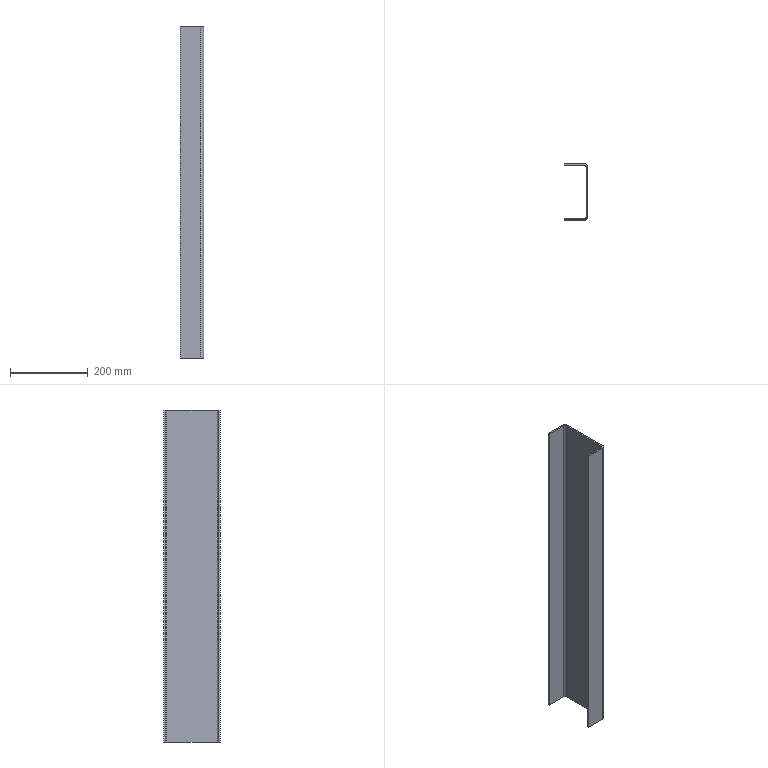Part | SolidWorks | features Extrusion 1 | 1 solid | 14 faces | box 60 x 145 x 854 mm | volume 860318 mm3 | plane 10 | cylinder 4 | commonest cylinder face diameters 8 x2 16 x2
STEP:
#1=CARTESIAN_POINT('',(-60.,-68.5,-427.));
#2=VERTEX_POINT('',#1);
#3=CARTESIAN_POINT('',(-60.,-72.5,-427.));
#4=VERTEX_POINT('',#3);
#5=CARTESIAN_POINT('',(-60.,-68.5,-427.));
#6=DIRECTION('',(0.,-1.,0.));
#7=VECTOR('',#6,1000.);
#8=LINE('',#5,#7);
#9=EDGE_CURVE('',#2,#4,#8,.T.);
#10=ORIENTED_EDGE('',*,*,#9,.T.);
#11=CARTESIAN_POINT('',(-60.,-72.5,427.));
#12=VERTEX_POINT('',#11);
#13=CARTESIAN_POINT('',(-60.,-72.5,427.));
#14=DIRECTION('',(0.,0.,-1.));
#15=VECTOR('',#14,1000.);
#16=LINE('',#13,#15);
#17=EDGE_CURVE('',#12,#4,#16,.T.);
#18=ORIENTED_EDGE('',*,*,#17,.F.);
#19=CARTESIAN_POINT('',(-60.,-68.5,427.));
#20=VERTEX_POINT('',#19);
#21=CARTESIAN_POINT('',(-60.,-68.5,427.));
#22=DIRECTION('',(0.,-1.,0.));
#23=VECTOR('',#22,1000.);
#24=LINE('',#21,#23);
#25=EDGE_CURVE('',#20,#12,#24,.T.);
#26=ORIENTED_EDGE('',*,*,#25,.F.);
#27=CARTESIAN_POINT('',(-60.,-68.5,427.));
#28=DIRECTION('',(0.,0.,-1.));
#29=VECTOR('',#28,1000.);
#30=LINE('',#27,#29);
#31=EDGE_CURVE('',#20,#2,#30,.T.);
#32=ORIENTED_EDGE('',*,*,#31,.T.);
#33=EDGE_LOOP('',(#10,#18,#26,#32));
#34=FACE_OUTER_BOUND('',#33,.T.);
#35=CARTESIAN_POINT('',(-60.,-68.5,427.));
#36=DIRECTION('',(1.,0.,0.));
#37=DIRECTION('',(0.,0.,-1.));
#38=AXIS2_PLACEMENT_3D('',#35,#36,#37);
#39=PLANE('',#38);
#40=ADVANCED_FACE('',(#34),#39,.F.);
#41=CARTESIAN_POINT('',(-8.,-72.5,-427.));
#42=VERTEX_POINT('',#41);
#43=CARTESIAN_POINT('',(-60.,-72.5,-427.));
#44=DIRECTION('',(1.,0.,0.));
#45=VECTOR('',#44,1000.);
#46=LINE('',#43,#45);
#47=EDGE_CURVE('',#4,#42,#46,.T.);
#48=ORIENTED_EDGE('',*,*,#47,.T.);
#49=CARTESIAN_POINT('',(-8.,-72.5,427.));
#50=VERTEX_POINT('',#49);
#51=CARTESIAN_POINT('',(-8.,-72.5,427.));
#52=DIRECTION('',(0.,0.,-1.));
#53=VECTOR('',#52,1000.);
#54=LINE('',#51,#53);
#55=EDGE_CURVE('',#50,#42,#54,.T.);
#56=ORIENTED_EDGE('',*,*,#55,.F.);
#57=CARTESIAN_POINT('',(-60.,-72.5,427.));
#58=DIRECTION('',(1.,0.,0.));
#59=VECTOR('',#58,1000.);
#60=LINE('',#57,#59);
#61=EDGE_CURVE('',#12,#50,#60,.T.);
#62=ORIENTED_EDGE('',*,*,#61,.F.);
#63=ORIENTED_EDGE('',*,*,#17,.T.);
#64=EDGE_LOOP('',(#48,#56,#62,#63));
#65=FACE_OUTER_BOUND('',#64,.T.);
#66=CARTESIAN_POINT('',(-60.,-72.5,427.));
#67=DIRECTION('',(0.,1.,0.));
#68=DIRECTION('',(0.,0.,1.));
#69=AXIS2_PLACEMENT_3D('',#66,#67,#68);
#70=PLANE('',#69);
#71=ADVANCED_FACE('',(#65),#70,.F.);
#72=CARTESIAN_POINT('',(0.,-64.5,-427.));
#73=VERTEX_POINT('',#72);
#74=CARTESIAN_POINT('',(-8.,-64.5,-427.));
#75=DIRECTION('',(0.,0.,1.));
#76=DIRECTION('',(1.,0.,0.));
#77=AXIS2_PLACEMENT_3D('',#74,#75,#76);
#78=CIRCLE('',#77,8.);
#79=EDGE_CURVE('',#42,#73,#78,.T.);
#80=ORIENTED_EDGE('',*,*,#79,.T.);
#81=CARTESIAN_POINT('',(0.,-64.5,427.));
#82=VERTEX_POINT('',#81);
#83=CARTESIAN_POINT('',(0.,-64.5,427.));
#84=DIRECTION('',(0.,0.,-1.));
#85=VECTOR('',#84,1000.);
#86=LINE('',#83,#85);
#87=EDGE_CURVE('',#82,#73,#86,.T.);
#88=ORIENTED_EDGE('',*,*,#87,.F.);
#89=CARTESIAN_POINT('',(-8.,-64.5,427.));
#90=DIRECTION('',(0.,0.,1.));
#91=DIRECTION('',(1.,0.,0.));
#92=AXIS2_PLACEMENT_3D('',#89,#90,#91);
#93=CIRCLE('',#92,8.);
#94=EDGE_CURVE('',#50,#82,#93,.T.);
#95=ORIENTED_EDGE('',*,*,#94,.F.);
#96=ORIENTED_EDGE('',*,*,#55,.T.);
#97=EDGE_LOOP('',(#80,#88,#95,#96));
#98=FACE_OUTER_BOUND('',#97,.T.);
#99=CARTESIAN_POINT('',(-8.,-64.5,427.));
#100=DIRECTION('',(0.,0.,-1.));
#101=DIRECTION('',(-1.,0.,0.));
#102=AXIS2_PLACEMENT_3D('',#99,#100,#101);
#103=CYLINDRICAL_SURFACE('',#102,8.);
#104=ADVANCED_FACE('',(#98),#103,.T.);
#105=CARTESIAN_POINT('',(0.,64.5,-427.));
#106=VERTEX_POINT('',#105);
#107=CARTESIAN_POINT('',(0.,-64.5,-427.));
#108=DIRECTION('',(0.,1.,0.));
#109=VECTOR('',#108,1000.);
#110=LINE('',#107,#109);
#111=EDGE_CURVE('',#73,#106,#110,.T.);
#112=ORIENTED_EDGE('',*,*,#111,.T.);
#113=CARTESIAN_POINT('',(0.,64.5,427.));
#114=VERTEX_POINT('',#113);
#115=CARTESIAN_POINT('',(0.,64.5,427.));
#116=DIRECTION('',(0.,0.,-1.));
#117=VECTOR('',#116,1000.);
#118=LINE('',#115,#117);
#119=EDGE_CURVE('',#114,#106,#118,.T.);
#120=ORIENTED_EDGE('',*,*,#119,.F.);
#121=CARTESIAN_POINT('',(0.,-64.5,427.));
#122=DIRECTION('',(0.,1.,0.));
#123=VECTOR('',#122,1000.);
#124=LINE('',#121,#123);
#125=EDGE_CURVE('',#82,#114,#124,.T.);
#126=ORIENTED_EDGE('',*,*,#125,.F.);
#127=ORIENTED_EDGE('',*,*,#87,.T.);
#128=EDGE_LOOP('',(#112,#120,#126,#127));
#129=FACE_OUTER_BOUND('',#128,.T.);
#130=CARTESIAN_POINT('',(0.,-64.5,427.));
#131=DIRECTION('',(-1.,0.,0.));
#132=DIRECTION('',(0.,0.,1.));
#133=AXIS2_PLACEMENT_3D('',#130,#131,#132);
#134=PLANE('',#133);
#135=ADVANCED_FACE('',(#129),#134,.F.);
#136=CARTESIAN_POINT('',(-8.,72.5,-427.));
#137=VERTEX_POINT('',#136);
#138=CARTESIAN_POINT('',(-8.,64.5,-427.));
#139=DIRECTION('',(0.,0.,1.));
#140=DIRECTION('',(1.,0.,0.));
#141=AXIS2_PLACEMENT_3D('',#138,#139,#140);
#142=CIRCLE('',#141,8.);
#143=EDGE_CURVE('',#106,#137,#142,.T.);
#144=ORIENTED_EDGE('',*,*,#143,.T.);
#145=CARTESIAN_POINT('',(-8.,72.5,427.));
#146=VERTEX_POINT('',#145);
#147=CARTESIAN_POINT('',(-8.,72.5,427.));
#148=DIRECTION('',(0.,0.,-1.));
#149=VECTOR('',#148,1000.);
#150=LINE('',#147,#149);
#151=EDGE_CURVE('',#146,#137,#150,.T.);
#152=ORIENTED_EDGE('',*,*,#151,.F.);
#153=CARTESIAN_POINT('',(-8.,64.5,427.));
#154=DIRECTION('',(0.,0.,1.));
#155=DIRECTION('',(1.,0.,0.));
#156=AXIS2_PLACEMENT_3D('',#153,#154,#155);
#157=CIRCLE('',#156,8.);
#158=EDGE_CURVE('',#114,#146,#157,.T.);
#159=ORIENTED_EDGE('',*,*,#158,.F.);
#160=ORIENTED_EDGE('',*,*,#119,.T.);
#161=EDGE_LOOP('',(#144,#152,#159,#160));
#162=FACE_OUTER_BOUND('',#161,.T.);
#163=CARTESIAN_POINT('',(-8.,64.5,427.));
#164=DIRECTION('',(0.,0.,-1.));
#165=DIRECTION('',(-1.,0.,0.));
#166=AXIS2_PLACEMENT_3D('',#163,#164,#165);
#167=CYLINDRICAL_SURFACE('',#166,8.);
#168=ADVANCED_FACE('',(#162),#167,.T.);
#169=CARTESIAN_POINT('',(-60.,72.5,-427.));
#170=VERTEX_POINT('',#169);
#171=CARTESIAN_POINT('',(-8.,72.5,-427.));
#172=DIRECTION('',(-1.,0.,0.));
#173=VECTOR('',#172,1000.);
#174=LINE('',#171,#173);
#175=EDGE_CURVE('',#137,#170,#174,.T.);
#176=ORIENTED_EDGE('',*,*,#175,.T.);
#177=CARTESIAN_POINT('',(-60.,72.5,427.));
#178=VERTEX_POINT('',#177);
#179=CARTESIAN_POINT('',(-60.,72.5,427.));
#180=DIRECTION('',(0.,0.,-1.));
#181=VECTOR('',#180,1000.);
#182=LINE('',#179,#181);
#183=EDGE_CURVE('',#178,#170,#182,.T.);
#184=ORIENTED_EDGE('',*,*,#183,.F.);
#185=CARTESIAN_POINT('',(-8.,72.5,427.));
#186=DIRECTION('',(-1.,0.,0.));
#187=VECTOR('',#186,1000.);
#188=LINE('',#185,#187);
#189=EDGE_CURVE('',#146,#178,#188,.T.);
#190=ORIENTED_EDGE('',*,*,#189,.F.);
#191=ORIENTED_EDGE('',*,*,#151,.T.);
#192=EDGE_LOOP('',(#176,#184,#190,#191));
#193=FACE_OUTER_BOUND('',#192,.T.);
#194=CARTESIAN_POINT('',(-8.,72.5,427.));
#195=DIRECTION('',(0.,-1.,0.));
#196=DIRECTION('',(1.,0.,0.));
#197=AXIS2_PLACEMENT_3D('',#194,#195,#196);
#198=PLANE('',#197);
#199=ADVANCED_FACE('',(#193),#198,.F.);
#200=CARTESIAN_POINT('',(-60.,68.5,-427.));
#201=VERTEX_POINT('',#200);
#202=CARTESIAN_POINT('',(-60.,72.5,-427.));
#203=DIRECTION('',(0.,-1.,0.));
#204=VECTOR('',#203,1000.);
#205=LINE('',#202,#204);
#206=EDGE_CURVE('',#170,#201,#205,.T.);
#207=ORIENTED_EDGE('',*,*,#206,.T.);
#208=CARTESIAN_POINT('',(-60.,68.5,427.));
#209=VERTEX_POINT('',#208);
#210=CARTESIAN_POINT('',(-60.,68.5,427.));
#211=DIRECTION('',(0.,0.,-1.));
#212=VECTOR('',#211,1000.);
#213=LINE('',#210,#212);
#214=EDGE_CURVE('',#209,#201,#213,.T.);
#215=ORIENTED_EDGE('',*,*,#214,.F.);
#216=CARTESIAN_POINT('',(-60.,72.5,427.));
#217=DIRECTION('',(0.,-1.,0.));
#218=VECTOR('',#217,1000.);
#219=LINE('',#216,#218);
#220=EDGE_CURVE('',#178,#209,#219,.T.);
#221=ORIENTED_EDGE('',*,*,#220,.F.);
#222=ORIENTED_EDGE('',*,*,#183,.T.);
#223=EDGE_LOOP('',(#207,#215,#221,#222));
#224=FACE_OUTER_BOUND('',#223,.T.);
#225=CARTESIAN_POINT('',(-60.,72.5,427.));
#226=DIRECTION('',(1.,0.,0.));
#227=DIRECTION('',(0.,0.,-1.));
#228=AXIS2_PLACEMENT_3D('',#225,#226,#227);
#229=PLANE('',#228);
#230=ADVANCED_FACE('',(#224),#229,.F.);
#231=CARTESIAN_POINT('',(-8.,68.5,-427.));
#232=VERTEX_POINT('',#231);
#233=CARTESIAN_POINT('',(-60.,68.5,-427.));
#234=DIRECTION('',(1.,0.,0.));
#235=VECTOR('',#234,1000.);
#236=LINE('',#233,#235);
#237=EDGE_CURVE('',#201,#232,#236,.T.);
#238=ORIENTED_EDGE('',*,*,#237,.T.);
#239=CARTESIAN_POINT('',(-8.,68.5,427.));
#240=VERTEX_POINT('',#239);
#241=CARTESIAN_POINT('',(-8.,68.5,427.));
#242=DIRECTION('',(0.,0.,-1.));
#243=VECTOR('',#242,1000.);
#244=LINE('',#241,#243);
#245=EDGE_CURVE('',#240,#232,#244,.T.);
#246=ORIENTED_EDGE('',*,*,#245,.F.);
#247=CARTESIAN_POINT('',(-60.,68.5,427.));
#248=DIRECTION('',(1.,0.,0.));
#249=VECTOR('',#248,1000.);
#250=LINE('',#247,#249);
#251=EDGE_CURVE('',#209,#240,#250,.T.);
#252=ORIENTED_EDGE('',*,*,#251,.F.);
#253=ORIENTED_EDGE('',*,*,#214,.T.);
#254=EDGE_LOOP('',(#238,#246,#252,#253));
#255=FACE_OUTER_BOUND('',#254,.T.);
#256=CARTESIAN_POINT('',(-60.,68.5,427.));
#257=DIRECTION('',(0.,1.,0.));
#258=DIRECTION('',(0.,0.,1.));
#259=AXIS2_PLACEMENT_3D('',#256,#257,#258);
#260=PLANE('',#259);
#261=ADVANCED_FACE('',(#255),#260,.F.);
#262=CARTESIAN_POINT('',(-4.,64.5,-427.));
#263=VERTEX_POINT('',#262);
#264=CARTESIAN_POINT('',(-8.,64.5,-427.));
#265=DIRECTION('',(0.,0.,-1.));
#266=DIRECTION('',(1.,0.,0.));
#267=AXIS2_PLACEMENT_3D('',#264,#265,#266);
#268=CIRCLE('',#267,4.);
#269=EDGE_CURVE('',#232,#263,#268,.T.);
#270=ORIENTED_EDGE('',*,*,#269,.T.);
#271=CARTESIAN_POINT('',(-4.,64.5,427.));
#272=VERTEX_POINT('',#271);
#273=CARTESIAN_POINT('',(-4.,64.5,427.));
#274=DIRECTION('',(0.,0.,-1.));
#275=VECTOR('',#274,1000.);
#276=LINE('',#273,#275);
#277=EDGE_CURVE('',#272,#263,#276,.T.);
#278=ORIENTED_EDGE('',*,*,#277,.F.);
#279=CARTESIAN_POINT('',(-8.,64.5,427.));
#280=DIRECTION('',(0.,0.,-1.));
#281=DIRECTION('',(1.,0.,0.));
#282=AXIS2_PLACEMENT_3D('',#279,#280,#281);
#283=CIRCLE('',#282,4.);
#284=EDGE_CURVE('',#240,#272,#283,.T.);
#285=ORIENTED_EDGE('',*,*,#284,.F.);
#286=ORIENTED_EDGE('',*,*,#245,.T.);
#287=EDGE_LOOP('',(#270,#278,#285,#286));
#288=FACE_OUTER_BOUND('',#287,.T.);
#289=CARTESIAN_POINT('',(-8.,64.5,427.));
#290=DIRECTION('',(0.,0.,-1.));
#291=DIRECTION('',(-1.,0.,0.));
#292=AXIS2_PLACEMENT_3D('',#289,#290,#291);
#293=CYLINDRICAL_SURFACE('',#292,4.);
#294=ADVANCED_FACE('',(#288),#293,.F.);
#295=CARTESIAN_POINT('',(-4.,-64.5,-427.));
#296=VERTEX_POINT('',#295);
#297=CARTESIAN_POINT('',(-4.,64.5,-427.));
#298=DIRECTION('',(0.,-1.,0.));
#299=VECTOR('',#298,1000.);
#300=LINE('',#297,#299);
#301=EDGE_CURVE('',#263,#296,#300,.T.);
#302=ORIENTED_EDGE('',*,*,#301,.T.);
#303=CARTESIAN_POINT('',(-4.,-64.5,427.));
#304=VERTEX_POINT('',#303);
#305=CARTESIAN_POINT('',(-4.,-64.5,427.));
#306=DIRECTION('',(0.,0.,-1.));
#307=VECTOR('',#306,1000.);
#308=LINE('',#305,#307);
#309=EDGE_CURVE('',#304,#296,#308,.T.);
#310=ORIENTED_EDGE('',*,*,#309,.F.);
#311=CARTESIAN_POINT('',(-4.,64.5,427.));
#312=DIRECTION('',(0.,-1.,0.));
#313=VECTOR('',#312,1000.);
#314=LINE('',#311,#313);
#315=EDGE_CURVE('',#272,#304,#314,.T.);
#316=ORIENTED_EDGE('',*,*,#315,.F.);
#317=ORIENTED_EDGE('',*,*,#277,.T.);
#318=EDGE_LOOP('',(#302,#310,#316,#317));
#319=FACE_OUTER_BOUND('',#318,.T.);
#320=CARTESIAN_POINT('',(-4.,64.5,427.));
#321=DIRECTION('',(1.,0.,0.));
#322=DIRECTION('',(0.,1.,0.));
#323=AXIS2_PLACEMENT_3D('',#320,#321,#322);
#324=PLANE('',#323);
#325=ADVANCED_FACE('',(#319),#324,.F.);
#326=CARTESIAN_POINT('',(-8.,-68.5,-427.));
#327=VERTEX_POINT('',#326);
#328=CARTESIAN_POINT('',(-8.,-64.5,-427.));
#329=DIRECTION('',(0.,0.,-1.));
#330=DIRECTION('',(1.,0.,0.));
#331=AXIS2_PLACEMENT_3D('',#328,#329,#330);
#332=CIRCLE('',#331,4.);
#333=EDGE_CURVE('',#296,#327,#332,.T.);
#334=ORIENTED_EDGE('',*,*,#333,.T.);
#335=CARTESIAN_POINT('',(-8.,-68.5,427.));
#336=VERTEX_POINT('',#335);
#337=CARTESIAN_POINT('',(-8.,-68.5,427.));
#338=DIRECTION('',(0.,0.,-1.));
#339=VECTOR('',#338,1000.);
#340=LINE('',#337,#339);
#341=EDGE_CURVE('',#336,#327,#340,.T.);
#342=ORIENTED_EDGE('',*,*,#341,.F.);
#343=CARTESIAN_POINT('',(-8.,-64.5,427.));
#344=DIRECTION('',(0.,0.,-1.));
#345=DIRECTION('',(1.,0.,0.));
#346=AXIS2_PLACEMENT_3D('',#343,#344,#345);
#347=CIRCLE('',#346,4.);
#348=EDGE_CURVE('',#304,#336,#347,.T.);
#349=ORIENTED_EDGE('',*,*,#348,.F.);
#350=ORIENTED_EDGE('',*,*,#309,.T.);
#351=EDGE_LOOP('',(#334,#342,#349,#350));
#352=FACE_OUTER_BOUND('',#351,.T.);
#353=CARTESIAN_POINT('',(-8.,-64.5,427.));
#354=DIRECTION('',(0.,0.,-1.));
#355=DIRECTION('',(-1.,0.,0.));
#356=AXIS2_PLACEMENT_3D('',#353,#354,#355);
#357=CYLINDRICAL_SURFACE('',#356,4.);
#358=ADVANCED_FACE('',(#352),#357,.F.);
#359=CARTESIAN_POINT('',(-8.,-68.5,-427.));
#360=DIRECTION('',(-1.,0.,0.));
#361=VECTOR('',#360,1000.);
#362=LINE('',#359,#361);
#363=EDGE_CURVE('',#327,#2,#362,.T.);
#364=ORIENTED_EDGE('',*,*,#363,.T.);
#365=ORIENTED_EDGE('',*,*,#31,.F.);
#366=CARTESIAN_POINT('',(-8.,-68.5,427.));
#367=DIRECTION('',(-1.,0.,0.));
#368=VECTOR('',#367,1000.);
#369=LINE('',#366,#368);
#370=EDGE_CURVE('',#336,#20,#369,.T.);
#371=ORIENTED_EDGE('',*,*,#370,.F.);
#372=ORIENTED_EDGE('',*,*,#341,.T.);
#373=EDGE_LOOP('',(#364,#365,#371,#372));
#374=FACE_OUTER_BOUND('',#373,.T.);
#375=CARTESIAN_POINT('',(-8.,-68.5,427.));
#376=DIRECTION('',(0.,-1.,0.));
#377=DIRECTION('',(0.,0.,-1.));
#378=AXIS2_PLACEMENT_3D('',#375,#376,#377);
#379=PLANE('',#378);
#380=ADVANCED_FACE('',(#374),#379,.F.);
#381=ORIENTED_EDGE('',*,*,#25,.T.);
#382=ORIENTED_EDGE('',*,*,#61,.T.);
#383=ORIENTED_EDGE('',*,*,#94,.T.);
#384=ORIENTED_EDGE('',*,*,#125,.T.);
#385=ORIENTED_EDGE('',*,*,#158,.T.);
#386=ORIENTED_EDGE('',*,*,#189,.T.);
#387=ORIENTED_EDGE('',*,*,#220,.T.);
#388=ORIENTED_EDGE('',*,*,#251,.T.);
#389=ORIENTED_EDGE('',*,*,#284,.T.);
#390=ORIENTED_EDGE('',*,*,#315,.T.);
#391=ORIENTED_EDGE('',*,*,#348,.T.);
#392=ORIENTED_EDGE('',*,*,#370,.T.);
#393=EDGE_LOOP('',(#381,#382,#383,#384,#385,#386,#387,#388,#389,#390,#391,#392));
#394=FACE_OUTER_BOUND('',#393,.T.);
#395=CARTESIAN_POINT('',(-8.,-64.5,427.));
#396=DIRECTION('',(0.,0.,1.));
#397=DIRECTION('',(1.,0.,0.));
#398=AXIS2_PLACEMENT_3D('',#395,#396,#397);
#399=PLANE('',#398);
#400=ADVANCED_FACE('',(#394),#399,.T.);
#401=ORIENTED_EDGE('',*,*,#9,.F.);
#402=ORIENTED_EDGE('',*,*,#363,.F.);
#403=ORIENTED_EDGE('',*,*,#333,.F.);
#404=ORIENTED_EDGE('',*,*,#301,.F.);
#405=ORIENTED_EDGE('',*,*,#269,.F.);
#406=ORIENTED_EDGE('',*,*,#237,.F.);
#407=ORIENTED_EDGE('',*,*,#206,.F.);
#408=ORIENTED_EDGE('',*,*,#175,.F.);
#409=ORIENTED_EDGE('',*,*,#143,.F.);
#410=ORIENTED_EDGE('',*,*,#111,.F.);
#411=ORIENTED_EDGE('',*,*,#79,.F.);
#412=ORIENTED_EDGE('',*,*,#47,.F.);
#413=EDGE_LOOP('',(#401,#402,#403,#404,#405,#406,#407,#408,#409,#410,#411,#412));
#414=FACE_OUTER_BOUND('',#413,.T.);
#415=CARTESIAN_POINT('',(-8.,-64.5,-427.));
#416=DIRECTION('',(0.,0.,1.));
#417=DIRECTION('',(1.,0.,0.));
#418=AXIS2_PLACEMENT_3D('',#415,#416,#417);
#419=PLANE('',#418);
#420=ADVANCED_FACE('',(#414),#419,.F.);
#421=CLOSED_SHELL('',(#40,#71,#104,#135,#168,#199,#230,#261,#294,#325,#358,#380,#400,#420));
#422=MANIFOLD_SOLID_BREP('',#421);
#423=CARTESIAN_POINT('',(0.,0.,0.));
#424=DIRECTION('',(0.,0.,1.));
#425=DIRECTION('',(1.,0.,0.));
#426=AXIS2_PLACEMENT_3D('',#423,#424,#425);
#427=(LENGTH_UNIT()NAMED_UNIT(*)SI_UNIT(.MILLI.,.METRE.));
#428=UNCERTAINTY_MEASURE_WITH_UNIT(LENGTH_MEASURE(0.00001),#427,'','');
#429=(NAMED_UNIT(*)PLANE_ANGLE_UNIT()SI_UNIT($,.RADIAN.));
#430=(NAMED_UNIT(*)SI_UNIT($,.STERADIAN.)SOLID_ANGLE_UNIT());
#431=(GEOMETRIC_REPRESENTATION_CONTEXT(3)GLOBAL_UNCERTAINTY_ASSIGNED_CONTEXT((#428))GLOBAL_UNIT_ASSIGNED_CONTEXT((#427,#429,#430))REPRESENTATION_CONTEXT('',''));
#432=ADVANCED_BREP_SHAPE_REPRESENTATION('',(#422,#426),#431);